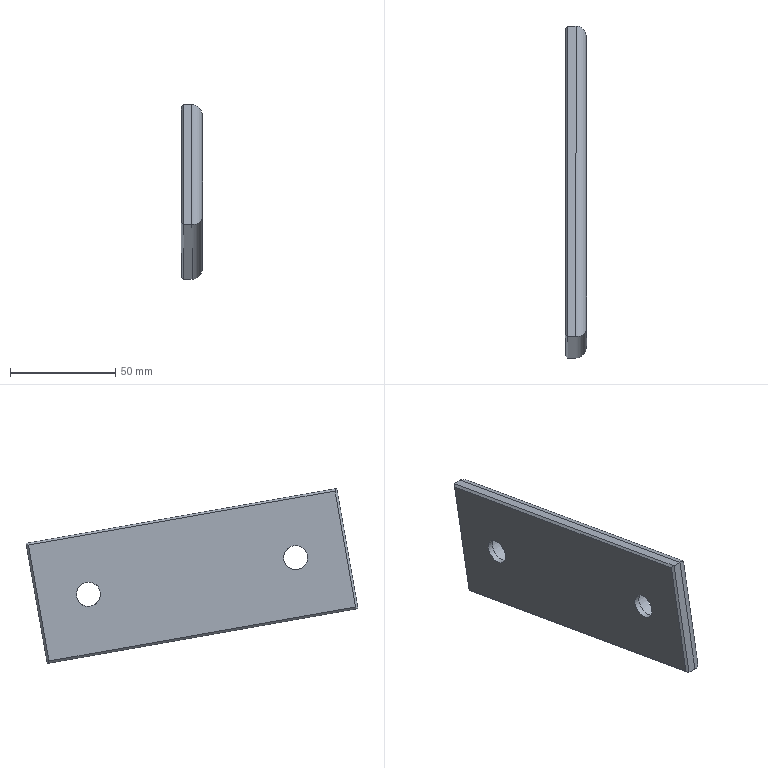Part | NX | features solid 2 | 1 solid | 20 faces | box 10 x 157.793 x 83.166 mm | volume 80537 mm3 | plane 12 | cylinder 8 | commonest cylinder face diameters 10 x4 11.5 x2 17.5 x2
STEP:
#1=CARTESIAN_POINT('',(875.238,-866.541,30.401));
#2=VERTEX_POINT('',#1);
#3=CARTESIAN_POINT('',(879.238,-866.541,30.401));
#4=VERTEX_POINT('',#3);
#5=CARTESIAN_POINT('',(874.238,-866.541,30.401));
#6=DIRECTION('',(1.,0.,0.));
#7=VECTOR('',#6,1000.);
#8=LINE('',#5,#7);
#9=EDGE_CURVE('',#2,#4,#8,.T.);
#10=ORIENTED_EDGE('',*,*,#9,.F.);
#11=CARTESIAN_POINT('',(875.238,-876.613,-26.718));
#12=VERTEX_POINT('',#11);
#13=CARTESIAN_POINT('',(875.238,-876.613,-26.718));
#14=DIRECTION('',(0.,-0.1736,-0.9848));
#15=VECTOR('',#14,1000.);
#16=LINE('',#13,#15);
#17=EDGE_CURVE('',#2,#12,#16,.T.);
#18=ORIENTED_EDGE('',*,*,#17,.T.);
#19=CARTESIAN_POINT('',(879.238,-876.613,-26.718));
#20=VERTEX_POINT('',#19);
#21=CARTESIAN_POINT('',(874.238,-876.613,-26.718));
#22=DIRECTION('',(1.,0.,0.));
#23=VECTOR('',#22,1000.);
#24=LINE('',#21,#23);
#25=EDGE_CURVE('',#12,#20,#24,.T.);
#26=ORIENTED_EDGE('',*,*,#25,.T.);
#27=CARTESIAN_POINT('',(879.238,-866.541,30.401));
#28=DIRECTION('',(0.,0.1736,0.9848));
#29=VECTOR('',#28,1000.);
#30=LINE('',#27,#29);
#31=EDGE_CURVE('',#20,#4,#30,.T.);
#32=ORIENTED_EDGE('',*,*,#31,.T.);
#33=EDGE_LOOP('',(#10,#18,#26,#32));
#34=FACE_BOUND('',#33,.T.);
#35=CARTESIAN_POINT('',(874.238,-876.613,-26.718));
#36=DIRECTION('',(0.,0.9848,-0.1736));
#37=DIRECTION('',(0.,0.1736,0.9848));
#38=AXIS2_PLACEMENT_3D('',#35,#36,#37);
#39=PLANE('',#38);
#40=ADVANCED_FACE('',(#34),#39,.F.);
#41=CARTESIAN_POINT('',(875.238,-718.82,4.353));
#42=VERTEX_POINT('',#41);
#43=CARTESIAN_POINT('',(879.238,-718.82,4.353));
#44=VERTEX_POINT('',#43);
#45=CARTESIAN_POINT('',(874.238,-718.82,4.353));
#46=DIRECTION('',(1.,0.,0.));
#47=VECTOR('',#46,1000.);
#48=LINE('',#45,#47);
#49=EDGE_CURVE('',#42,#44,#48,.T.);
#50=ORIENTED_EDGE('',*,*,#49,.F.);
#51=CARTESIAN_POINT('',(875.238,-841.921,26.06));
#52=DIRECTION('',(0.,-0.9848,0.1736));
#53=VECTOR('',#52,1000.);
#54=LINE('',#51,#53);
#55=EDGE_CURVE('',#42,#2,#54,.T.);
#56=ORIENTED_EDGE('',*,*,#55,.T.);
#57=ORIENTED_EDGE('',*,*,#9,.T.);
#58=CARTESIAN_POINT('',(879.238,-743.44,8.695));
#59=DIRECTION('',(0.,0.9848,-0.1736));
#60=VECTOR('',#59,1000.);
#61=LINE('',#58,#60);
#62=EDGE_CURVE('',#4,#44,#61,.T.);
#63=ORIENTED_EDGE('',*,*,#62,.T.);
#64=EDGE_LOOP('',(#50,#56,#57,#63));
#65=FACE_BOUND('',#64,.T.);
#66=CARTESIAN_POINT('',(874.238,-841.921,26.06));
#67=DIRECTION('',(0.,-0.1736,-0.9848));
#68=DIRECTION('',(0.,0.9848,-0.1736));
#69=AXIS2_PLACEMENT_3D('',#66,#67,#68);
#70=PLANE('',#69);
#71=ADVANCED_FACE('',(#65),#70,.F.);
#72=CARTESIAN_POINT('',(875.238,-728.892,-52.765));
#73=VERTEX_POINT('',#72);
#74=CARTESIAN_POINT('',(879.238,-728.892,-52.765));
#75=VERTEX_POINT('',#74);
#76=CARTESIAN_POINT('',(874.238,-728.892,-52.765));
#77=DIRECTION('',(1.,0.,0.));
#78=VECTOR('',#77,1000.);
#79=LINE('',#76,#78);
#80=EDGE_CURVE('',#73,#75,#79,.T.);
#81=ORIENTED_EDGE('',*,*,#80,.F.);
#82=CARTESIAN_POINT('',(875.238,-718.82,4.353));
#83=DIRECTION('',(0.,0.1736,0.9848));
#84=VECTOR('',#83,1000.);
#85=LINE('',#82,#84);
#86=EDGE_CURVE('',#73,#42,#85,.T.);
#87=ORIENTED_EDGE('',*,*,#86,.T.);
#88=ORIENTED_EDGE('',*,*,#49,.T.);
#89=CARTESIAN_POINT('',(879.238,-728.892,-52.765));
#90=DIRECTION('',(0.,-0.1736,-0.9848));
#91=VECTOR('',#90,1000.);
#92=LINE('',#89,#91);
#93=EDGE_CURVE('',#44,#75,#92,.T.);
#94=ORIENTED_EDGE('',*,*,#93,.T.);
#95=EDGE_LOOP('',(#81,#87,#88,#94));
#96=FACE_BOUND('',#95,.T.);
#97=CARTESIAN_POINT('',(874.238,-718.82,4.353));
#98=DIRECTION('',(0.,-0.9848,0.1736));
#99=DIRECTION('',(0.,-0.1736,-0.9848));
#100=AXIS2_PLACEMENT_3D('',#97,#98,#99);
#101=PLANE('',#100);
#102=ADVANCED_FACE('',(#96),#101,.F.);
#103=ORIENTED_EDGE('',*,*,#25,.F.);
#104=CARTESIAN_POINT('',(875.238,-753.512,-48.424));
#105=DIRECTION('',(0.,0.9848,-0.1736));
#106=VECTOR('',#105,1000.);
#107=LINE('',#104,#106);
#108=EDGE_CURVE('',#12,#73,#107,.T.);
#109=ORIENTED_EDGE('',*,*,#108,.T.);
#110=ORIENTED_EDGE('',*,*,#80,.T.);
#111=CARTESIAN_POINT('',(879.238,-851.992,-31.059));
#112=DIRECTION('',(0.,-0.9848,0.1736));
#113=VECTOR('',#112,1000.);
#114=LINE('',#111,#113);
#115=EDGE_CURVE('',#75,#20,#114,.T.);
#116=ORIENTED_EDGE('',*,*,#115,.T.);
#117=EDGE_LOOP('',(#103,#109,#110,#116));
#118=FACE_BOUND('',#117,.T.);
#119=CARTESIAN_POINT('',(874.238,-753.512,-48.424));
#120=DIRECTION('',(0.,0.1736,0.9848));
#121=DIRECTION('',(0.,-0.9848,0.1736));
#122=AXIS2_PLACEMENT_3D('',#119,#120,#121);
#123=PLANE('',#122);
#124=ADVANCED_FACE('',(#118),#123,.F.);
#125=CARTESIAN_POINT('',(874.238,-875.454,-25.907));
#126=VERTEX_POINT('',#125);
#127=CARTESIAN_POINT('',(874.238,-865.73,29.242));
#128=VERTEX_POINT('',#127);
#129=CARTESIAN_POINT('',(874.238,-875.628,-26.892));
#130=DIRECTION('',(0.,-0.1736,-0.9848));
#131=VECTOR('',#130,1000.);
#132=LINE('',#129,#131);
#133=EDGE_CURVE('',#126,#128,#132,.F.);
#134=ORIENTED_EDGE('',*,*,#133,.T.);
#135=CARTESIAN_POINT('',(874.238,-719.978,3.542));
#136=VERTEX_POINT('',#135);
#137=CARTESIAN_POINT('',(874.238,-842.095,25.075));
#138=DIRECTION('',(0.,0.9848,-0.1736));
#139=VECTOR('',#138,1000.);
#140=LINE('',#137,#139);
#141=EDGE_CURVE('',#128,#136,#140,.T.);
#142=ORIENTED_EDGE('',*,*,#141,.T.);
#143=CARTESIAN_POINT('',(874.238,-729.703,-51.607));
#144=VERTEX_POINT('',#143);
#145=CARTESIAN_POINT('',(874.238,-729.876,-52.592));
#146=DIRECTION('',(0.,0.1736,0.9848));
#147=VECTOR('',#146,1000.);
#148=LINE('',#145,#147);
#149=EDGE_CURVE('',#136,#144,#148,.F.);
#150=ORIENTED_EDGE('',*,*,#149,.T.);
#151=CARTESIAN_POINT('',(874.238,-851.819,-30.075));
#152=DIRECTION('',(0.,-0.9848,0.1736));
#153=VECTOR('',#152,1000.);
#154=LINE('',#151,#153);
#155=EDGE_CURVE('',#144,#126,#154,.T.);
#156=ORIENTED_EDGE('',*,*,#155,.T.);
#157=EDGE_LOOP('',(#134,#142,#150,#156));
#158=FACE_BOUND('',#157,.T.);
#159=CARTESIAN_POINT('',(874.238,-748.476,-25.615));
#160=VERTEX_POINT('',#159);
#161=CARTESIAN_POINT('',(874.238,-748.476,-19.865));
#162=DIRECTION('',(1.,0.,0.));
#163=DIRECTION('',(0.,0.,-1.));
#164=AXIS2_PLACEMENT_3D('',#161,#162,#163);
#165=CIRCLE('',#164,5.75);
#166=EDGE_CURVE('',#160,#160,#165,.T.);
#167=ORIENTED_EDGE('',*,*,#166,.T.);
#168=EDGE_LOOP('',(#167));
#169=FACE_BOUND('',#168,.T.);
#170=CARTESIAN_POINT('',(874.238,-846.957,-8.25));
#171=VERTEX_POINT('',#170);
#172=CARTESIAN_POINT('',(874.238,-846.957,-2.5));
#173=DIRECTION('',(1.,0.,0.));
#174=DIRECTION('',(0.,0.,-1.));
#175=AXIS2_PLACEMENT_3D('',#172,#173,#174);
#176=CIRCLE('',#175,5.75);
#177=EDGE_CURVE('',#171,#171,#176,.T.);
#178=ORIENTED_EDGE('',*,*,#177,.T.);
#179=EDGE_LOOP('',(#178));
#180=FACE_BOUND('',#179,.T.);
#181=CARTESIAN_POINT('',(874.238,-851.992,-31.059));
#182=DIRECTION('',(1.,0.,0.));
#183=DIRECTION('',(0.,0.9848,-0.1736));
#184=AXIS2_PLACEMENT_3D('',#181,#182,#183);
#185=PLANE('',#184);
#186=ADVANCED_FACE('',(#158,#169,#180),#185,.F.);
#187=CARTESIAN_POINT('',(884.238,-732.947,-46.973));
#188=VERTEX_POINT('',#187);
#189=CARTESIAN_POINT('',(884.238,-724.612,0.2977));
#190=VERTEX_POINT('',#189);
#191=CARTESIAN_POINT('',(884.238,-723.744,5.222));
#192=DIRECTION('',(0.,-0.1736,-0.9848));
#193=VECTOR('',#192,1000.);
#194=LINE('',#191,#193);
#195=EDGE_CURVE('',#188,#190,#194,.F.);
#196=ORIENTED_EDGE('',*,*,#195,.T.);
#197=CARTESIAN_POINT('',(884.238,-862.485,24.608));
#198=VERTEX_POINT('',#197);
#199=CARTESIAN_POINT('',(884.238,-842.789,21.135));
#200=DIRECTION('',(0.,0.9848,-0.1736));
#201=VECTOR('',#200,1000.);
#202=LINE('',#199,#201);
#203=EDGE_CURVE('',#190,#198,#202,.F.);
#204=ORIENTED_EDGE('',*,*,#203,.T.);
#205=CARTESIAN_POINT('',(884.238,-870.82,-22.662));
#206=VERTEX_POINT('',#205);
#207=CARTESIAN_POINT('',(884.238,-871.689,-27.586));
#208=DIRECTION('',(0.,0.1736,0.9848));
#209=VECTOR('',#208,1000.);
#210=LINE('',#207,#209);
#211=EDGE_CURVE('',#198,#206,#210,.F.);
#212=ORIENTED_EDGE('',*,*,#211,.T.);
#213=CARTESIAN_POINT('',(884.238,-752.643,-43.5));
#214=DIRECTION('',(0.,-0.9848,0.1736));
#215=VECTOR('',#214,1000.);
#216=LINE('',#213,#215);
#217=EDGE_CURVE('',#206,#188,#216,.F.);
#218=ORIENTED_EDGE('',*,*,#217,.T.);
#219=EDGE_LOOP('',(#196,#204,#212,#218));
#220=FACE_BOUND('',#219,.T.);
#221=CARTESIAN_POINT('',(884.238,-748.476,-28.615));
#222=VERTEX_POINT('',#221);
#223=CARTESIAN_POINT('',(884.238,-748.476,-19.865));
#224=DIRECTION('',(1.,0.,0.));
#225=DIRECTION('',(0.,0.,-1.));
#226=AXIS2_PLACEMENT_3D('',#223,#224,#225);
#227=CIRCLE('',#226,8.75);
#228=EDGE_CURVE('',#222,#222,#227,.F.);
#229=ORIENTED_EDGE('',*,*,#228,.T.);
#230=EDGE_LOOP('',(#229));
#231=FACE_BOUND('',#230,.T.);
#232=CARTESIAN_POINT('',(884.238,-846.957,-11.25));
#233=VERTEX_POINT('',#232);
#234=CARTESIAN_POINT('',(884.238,-846.957,-2.5));
#235=DIRECTION('',(1.,0.,0.));
#236=DIRECTION('',(0.,0.,-1.));
#237=AXIS2_PLACEMENT_3D('',#234,#235,#236);
#238=CIRCLE('',#237,8.75);
#239=EDGE_CURVE('',#233,#233,#238,.F.);
#240=ORIENTED_EDGE('',*,*,#239,.T.);
#241=EDGE_LOOP('',(#240));
#242=FACE_BOUND('',#241,.T.);
#243=CARTESIAN_POINT('',(884.238,-851.992,-31.059));
#244=DIRECTION('',(1.,0.,0.));
#245=DIRECTION('',(0.,0.9848,-0.1736));
#246=AXIS2_PLACEMENT_3D('',#243,#244,#245);
#247=PLANE('',#246);
#248=ADVANCED_FACE('',(#220,#231,#242),#247,.T.);
#249=CARTESIAN_POINT('',(876.938,-852.619,-1.501));
#250=VERTEX_POINT('',#249);
#251=CARTESIAN_POINT('',(876.938,-846.957,-2.5));
#252=DIRECTION('',(-1.,0.,0.));
#253=DIRECTION('',(0.,-0.9848,0.1736));
#254=AXIS2_PLACEMENT_3D('',#251,#252,#253);
#255=CIRCLE('',#254,5.75);
#256=EDGE_CURVE('',#250,#250,#255,.T.);
#257=ORIENTED_EDGE('',*,*,#256,.F.);
#258=EDGE_LOOP('',(#257));
#259=FACE_BOUND('',#258,.T.);
#260=ORIENTED_EDGE('',*,*,#177,.F.);
#261=EDGE_LOOP('',(#260));
#262=FACE_BOUND('',#261,.T.);
#263=CARTESIAN_POINT('',(834.238,-846.957,-2.5));
#264=DIRECTION('',(-1.,0.,0.));
#265=DIRECTION('',(0.,-0.9848,0.1736));
#266=AXIS2_PLACEMENT_3D('',#263,#264,#265);
#267=CYLINDRICAL_SURFACE('',#266,5.75);
#268=ADVANCED_FACE('',(#259,#262),#267,.F.);
#269=ORIENTED_EDGE('',*,*,#256,.T.);
#270=EDGE_LOOP('',(#269));
#271=FACE_BOUND('',#270,.T.);
#272=CARTESIAN_POINT('',(876.938,-855.574,-0.9805));
#273=VERTEX_POINT('',#272);
#274=CARTESIAN_POINT('',(876.938,-846.957,-2.5));
#275=DIRECTION('',(-1.,0.,0.));
#276=DIRECTION('',(0.,-0.9848,0.1736));
#277=AXIS2_PLACEMENT_3D('',#274,#275,#276);
#278=CIRCLE('',#277,8.75);
#279=EDGE_CURVE('',#273,#273,#278,.T.);
#280=ORIENTED_EDGE('',*,*,#279,.F.);
#281=EDGE_LOOP('',(#280));
#282=FACE_BOUND('',#281,.T.);
#283=CARTESIAN_POINT('',(876.938,-846.957,-2.5));
#284=DIRECTION('',(-1.,0.,0.));
#285=DIRECTION('',(0.,-0.9848,0.1736));
#286=AXIS2_PLACEMENT_3D('',#283,#284,#285);
#287=PLANE('',#286);
#288=ADVANCED_FACE('',(#271,#282),#287,.F.);
#289=ORIENTED_EDGE('',*,*,#279,.T.);
#290=EDGE_LOOP('',(#289));
#291=FACE_BOUND('',#290,.T.);
#292=ORIENTED_EDGE('',*,*,#239,.F.);
#293=EDGE_LOOP('',(#292));
#294=FACE_BOUND('',#293,.T.);
#295=CARTESIAN_POINT('',(884.238,-846.957,-2.5));
#296=DIRECTION('',(-1.,0.,0.));
#297=DIRECTION('',(0.,-0.9848,0.1736));
#298=AXIS2_PLACEMENT_3D('',#295,#296,#297);
#299=CYLINDRICAL_SURFACE('',#298,8.75);
#300=ADVANCED_FACE('',(#291,#294),#299,.F.);
#301=CARTESIAN_POINT('',(876.938,-754.139,-18.866));
#302=VERTEX_POINT('',#301);
#303=CARTESIAN_POINT('',(876.938,-748.476,-19.865));
#304=DIRECTION('',(-1.,0.,0.));
#305=DIRECTION('',(0.,-0.9848,0.1736));
#306=AXIS2_PLACEMENT_3D('',#303,#304,#305);
#307=CIRCLE('',#306,5.75);
#308=EDGE_CURVE('',#302,#302,#307,.T.);
#309=ORIENTED_EDGE('',*,*,#308,.F.);
#310=EDGE_LOOP('',(#309));
#311=FACE_BOUND('',#310,.T.);
#312=ORIENTED_EDGE('',*,*,#166,.F.);
#313=EDGE_LOOP('',(#312));
#314=FACE_BOUND('',#313,.T.);
#315=CARTESIAN_POINT('',(834.238,-748.476,-19.865));
#316=DIRECTION('',(-1.,0.,0.));
#317=DIRECTION('',(0.,-0.9848,0.1736));
#318=AXIS2_PLACEMENT_3D('',#315,#316,#317);
#319=CYLINDRICAL_SURFACE('',#318,5.75);
#320=ADVANCED_FACE('',(#311,#314),#319,.F.);
#321=ORIENTED_EDGE('',*,*,#308,.T.);
#322=EDGE_LOOP('',(#321));
#323=FACE_BOUND('',#322,.T.);
#324=CARTESIAN_POINT('',(876.938,-757.093,-18.345));
#325=VERTEX_POINT('',#324);
#326=CARTESIAN_POINT('',(876.938,-748.476,-19.865));
#327=DIRECTION('',(-1.,0.,0.));
#328=DIRECTION('',(0.,-0.9848,0.1736));
#329=AXIS2_PLACEMENT_3D('',#326,#327,#328);
#330=CIRCLE('',#329,8.75);
#331=EDGE_CURVE('',#325,#325,#330,.T.);
#332=ORIENTED_EDGE('',*,*,#331,.F.);
#333=EDGE_LOOP('',(#332));
#334=FACE_BOUND('',#333,.T.);
#335=CARTESIAN_POINT('',(876.938,-748.476,-19.865));
#336=DIRECTION('',(-1.,0.,0.));
#337=DIRECTION('',(0.,-0.9848,0.1736));
#338=AXIS2_PLACEMENT_3D('',#335,#336,#337);
#339=PLANE('',#338);
#340=ADVANCED_FACE('',(#323,#334),#339,.F.);
#341=ORIENTED_EDGE('',*,*,#331,.T.);
#342=EDGE_LOOP('',(#341));
#343=FACE_BOUND('',#342,.T.);
#344=ORIENTED_EDGE('',*,*,#228,.F.);
#345=EDGE_LOOP('',(#344));
#346=FACE_BOUND('',#345,.T.);
#347=CARTESIAN_POINT('',(884.238,-748.476,-19.865));
#348=DIRECTION('',(-1.,0.,0.));
#349=DIRECTION('',(0.,-0.9848,0.1736));
#350=AXIS2_PLACEMENT_3D('',#347,#348,#349);
#351=CYLINDRICAL_SURFACE('',#350,8.75);
#352=ADVANCED_FACE('',(#343,#346),#351,.F.);
#353=CARTESIAN_POINT('',(879.238,-732.947,-46.973));
#354=DIRECTION('',(0.,0.8192,0.5736));
#355=DIRECTION('',(0.,-0.5736,0.8192));
#356=AXIS2_PLACEMENT_3D('',#353,#354,#355);
#357=ELLIPSE('',#356,7.071,5.);
#358=EDGE_CURVE('',#188,#75,#357,.T.);
#359=ORIENTED_EDGE('',*,*,#358,.F.);
#360=ORIENTED_EDGE('',*,*,#217,.F.);
#361=CARTESIAN_POINT('',(879.238,-870.82,-22.662));
#362=DIRECTION('',(0.,0.5736,-0.8192));
#363=DIRECTION('',(0.,-0.8192,-0.5736));
#364=AXIS2_PLACEMENT_3D('',#361,#362,#363);
#365=ELLIPSE('',#364,7.071,5.);
#366=EDGE_CURVE('',#20,#206,#365,.F.);
#367=ORIENTED_EDGE('',*,*,#366,.F.);
#368=ORIENTED_EDGE('',*,*,#115,.F.);
#369=EDGE_LOOP('',(#359,#360,#367,#368));
#370=FACE_BOUND('',#369,.T.);
#371=CARTESIAN_POINT('',(879.238,-752.643,-43.5));
#372=DIRECTION('',(0.,0.9848,-0.1736));
#373=DIRECTION('',(0.,0.1736,0.9848));
#374=AXIS2_PLACEMENT_3D('',#371,#372,#373);
#375=CYLINDRICAL_SURFACE('',#374,5.);
#376=ADVANCED_FACE('',(#370),#375,.T.);
#377=ORIENTED_EDGE('',*,*,#366,.T.);
#378=ORIENTED_EDGE('',*,*,#211,.F.);
#379=CARTESIAN_POINT('',(879.238,-862.485,24.608));
#380=DIRECTION('',(0.,-0.8192,-0.5736));
#381=DIRECTION('',(0.,-0.5736,0.8192));
#382=AXIS2_PLACEMENT_3D('',#379,#380,#381);
#383=ELLIPSE('',#382,7.071,5.);
#384=EDGE_CURVE('',#4,#198,#383,.F.);
#385=ORIENTED_EDGE('',*,*,#384,.F.);
#386=ORIENTED_EDGE('',*,*,#31,.F.);
#387=EDGE_LOOP('',(#377,#378,#385,#386));
#388=FACE_BOUND('',#387,.T.);
#389=CARTESIAN_POINT('',(879.238,-871.689,-27.586));
#390=DIRECTION('',(0.,-0.1736,-0.9848));
#391=DIRECTION('',(0.,0.9848,-0.1736));
#392=AXIS2_PLACEMENT_3D('',#389,#390,#391);
#393=CYLINDRICAL_SURFACE('',#392,5.);
#394=ADVANCED_FACE('',(#388),#393,.T.);
#395=ORIENTED_EDGE('',*,*,#358,.T.);
#396=ORIENTED_EDGE('',*,*,#93,.F.);
#397=CARTESIAN_POINT('',(879.238,-724.612,0.2977));
#398=DIRECTION('',(0.,-0.5736,0.8192));
#399=DIRECTION('',(0.,-0.8192,-0.5736));
#400=AXIS2_PLACEMENT_3D('',#397,#398,#399);
#401=ELLIPSE('',#400,7.071,5.);
#402=EDGE_CURVE('',#190,#44,#401,.T.);
#403=ORIENTED_EDGE('',*,*,#402,.F.);
#404=ORIENTED_EDGE('',*,*,#195,.F.);
#405=EDGE_LOOP('',(#395,#396,#403,#404));
#406=FACE_BOUND('',#405,.T.);
#407=CARTESIAN_POINT('',(879.238,-723.744,5.222));
#408=DIRECTION('',(0.,0.1736,0.9848));
#409=DIRECTION('',(0.,-0.9848,0.1736));
#410=AXIS2_PLACEMENT_3D('',#407,#408,#409);
#411=CYLINDRICAL_SURFACE('',#410,5.);
#412=ADVANCED_FACE('',(#406),#411,.T.);
#413=ORIENTED_EDGE('',*,*,#384,.T.);
#414=ORIENTED_EDGE('',*,*,#203,.F.);
#415=ORIENTED_EDGE('',*,*,#402,.T.);
#416=ORIENTED_EDGE('',*,*,#62,.F.);
#417=EDGE_LOOP('',(#413,#414,#415,#416));
#418=FACE_BOUND('',#417,.T.);
#419=CARTESIAN_POINT('',(879.238,-842.789,21.135));
#420=DIRECTION('',(0.,-0.9848,0.1736));
#421=DIRECTION('',(0.,-0.1736,-0.9848));
#422=AXIS2_PLACEMENT_3D('',#419,#420,#421);
#423=CYLINDRICAL_SURFACE('',#422,5.);
#424=ADVANCED_FACE('',(#418),#423,.T.);
#425=CARTESIAN_POINT('',(874.571,-729.432,-51.993));
#426=DIRECTION('',(-0.5774,-0.4683,0.6688));
#427=VECTOR('',#426,1000.);
#428=LINE('',#425,#427);
#429=EDGE_CURVE('',#73,#144,#428,.T.);
#430=ORIENTED_EDGE('',*,*,#429,.F.);
#431=ORIENTED_EDGE('',*,*,#108,.F.);
#432=CARTESIAN_POINT('',(874.571,-875.84,-26.177));
#433=DIRECTION('',(0.5774,-0.6688,-0.4683));
#434=VECTOR('',#433,1000.);
#435=LINE('',#432,#434);
#436=EDGE_CURVE('',#126,#12,#435,.T.);
#437=ORIENTED_EDGE('',*,*,#436,.F.);
#438=ORIENTED_EDGE('',*,*,#155,.F.);
#439=EDGE_LOOP('',(#430,#431,#437,#438));
#440=FACE_BOUND('',#439,.T.);
#441=CARTESIAN_POINT('',(874.238,-851.819,-30.075));
#442=DIRECTION('',(0.7071,0.1228,0.6964));
#443=DIRECTION('',(0.7071,-0.1228,-0.6964));
#444=AXIS2_PLACEMENT_3D('',#441,#442,#443);
#445=PLANE('',#444);
#446=ADVANCED_FACE('',(#440),#445,.F.);
#447=ORIENTED_EDGE('',*,*,#436,.T.);
#448=ORIENTED_EDGE('',*,*,#17,.F.);
#449=CARTESIAN_POINT('',(866.238,-859.241,19.975));
#450=DIRECTION('',(0.5774,-0.4683,0.6688));
#451=VECTOR('',#450,1000.);
#452=LINE('',#449,#451);
#453=EDGE_CURVE('',#128,#2,#452,.T.);
#454=ORIENTED_EDGE('',*,*,#453,.F.);
#455=ORIENTED_EDGE('',*,*,#133,.F.);
#456=EDGE_LOOP('',(#447,#448,#454,#455));
#457=FACE_BOUND('',#456,.T.);
#458=CARTESIAN_POINT('',(874.238,-875.628,-26.892));
#459=DIRECTION('',(0.7071,0.6964,-0.1228));
#460=DIRECTION('',(-0.7071,0.6964,-0.1228));
#461=AXIS2_PLACEMENT_3D('',#458,#459,#460);
#462=PLANE('',#461);
#463=ADVANCED_FACE('',(#457),#462,.F.);
#464=ORIENTED_EDGE('',*,*,#429,.T.);
#465=ORIENTED_EDGE('',*,*,#149,.F.);
#466=CARTESIAN_POINT('',(832.904,-767.861,-29.986));
#467=DIRECTION('',(-0.5774,-0.6688,-0.4683));
#468=VECTOR('',#467,1000.);
#469=LINE('',#466,#468);
#470=EDGE_CURVE('',#42,#136,#469,.T.);
#471=ORIENTED_EDGE('',*,*,#470,.F.);
#472=ORIENTED_EDGE('',*,*,#86,.F.);
#473=EDGE_LOOP('',(#464,#465,#471,#472));
#474=FACE_BOUND('',#473,.T.);
#475=CARTESIAN_POINT('',(874.238,-729.876,-52.592));
#476=DIRECTION('',(0.7071,-0.6964,0.1228));
#477=DIRECTION('',(0.7071,0.6964,-0.1228));
#478=AXIS2_PLACEMENT_3D('',#475,#476,#477);
#479=PLANE('',#478);
#480=ADVANCED_FACE('',(#474),#479,.F.);
#481=ORIENTED_EDGE('',*,*,#453,.T.);
#482=ORIENTED_EDGE('',*,*,#55,.F.);
#483=ORIENTED_EDGE('',*,*,#470,.T.);
#484=ORIENTED_EDGE('',*,*,#141,.F.);
#485=EDGE_LOOP('',(#481,#482,#483,#484));
#486=FACE_BOUND('',#485,.T.);
#487=CARTESIAN_POINT('',(874.238,-842.095,25.075));
#488=DIRECTION('',(0.7071,-0.1228,-0.6964));
#489=DIRECTION('',(-0.7071,-0.1228,-0.6964));
#490=AXIS2_PLACEMENT_3D('',#487,#488,#489);
#491=PLANE('',#490);
#492=ADVANCED_FACE('',(#486),#491,.F.);
#493=CLOSED_SHELL('',(#40,#71,#102,#124,#186,#248,#268,#288,#300,#320,#340,#352,#376,#394,#412,#424,#446,#463,#480,#492));
#494=MANIFOLD_SOLID_BREP('',#493);
#495=(LENGTH_UNIT()NAMED_UNIT(*)SI_UNIT(.MILLI.,.METRE.));
#496=UNCERTAINTY_MEASURE_WITH_UNIT(LENGTH_MEASURE(0.00001),#495,'','');
#497=(NAMED_UNIT(*)PLANE_ANGLE_UNIT()SI_UNIT($,.RADIAN.));
#498=(NAMED_UNIT(*)SI_UNIT($,.STERADIAN.)SOLID_ANGLE_UNIT());
#499=(GEOMETRIC_REPRESENTATION_CONTEXT(3)GLOBAL_UNCERTAINTY_ASSIGNED_CONTEXT((#496))GLOBAL_UNIT_ASSIGNED_CONTEXT((#495,#497,#498))REPRESENTATION_CONTEXT('',''));
#500=ADVANCED_BREP_SHAPE_REPRESENTATION('',(#494),#499);